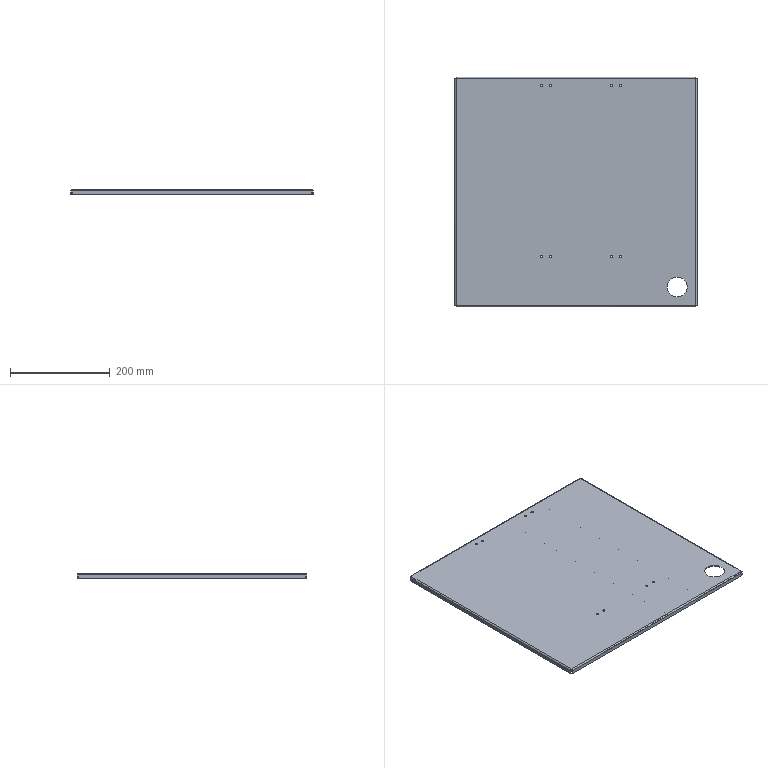Part | STEP file | 11-FG-JX01411 | 1 solid | 65 faces | box 485 x 460 x 10 mm | volume 675418 mm3 | plane 29 | cylinder 28 | spline 8 | commonest cylinder face diameters 4.2 x16 1.473 x6 5.473 x4 40 x2